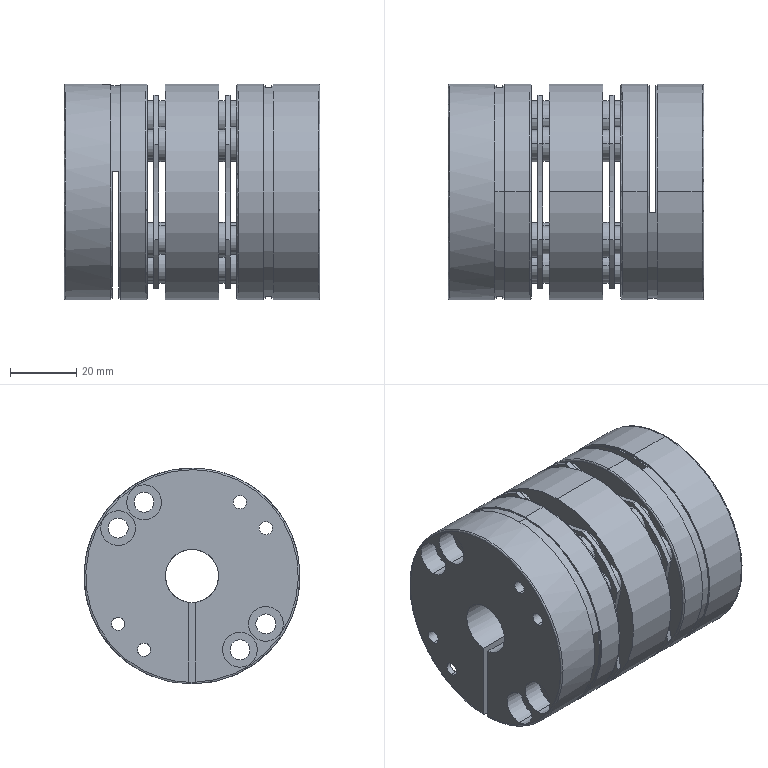Part | STEP file | 0245_Z_029_CPSWC65-16-16_1 | 1 solid | 225 faces | box 77 x 65 x 65 mm | volume 176037 mm3 | cylinder 172 | plane 40 | spline 9 | cone 4 | commonest cylinder face diameters 10.5 x48 8.5 x32 4 x20 65 x18 6 x16 100 x10